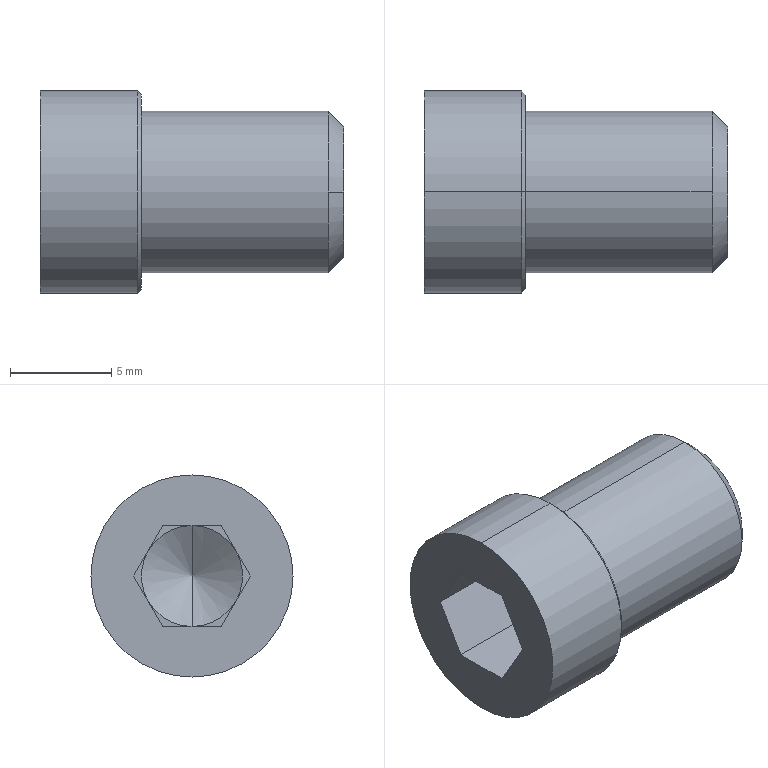Part | STEP file | 1 solid | 25 faces | box 15 x 10 x 10 mm | volume 791.764 mm3 | plane 15 | cone 6 | cylinder 4 | commonest cylinder face diameters 8 x2 10 x2